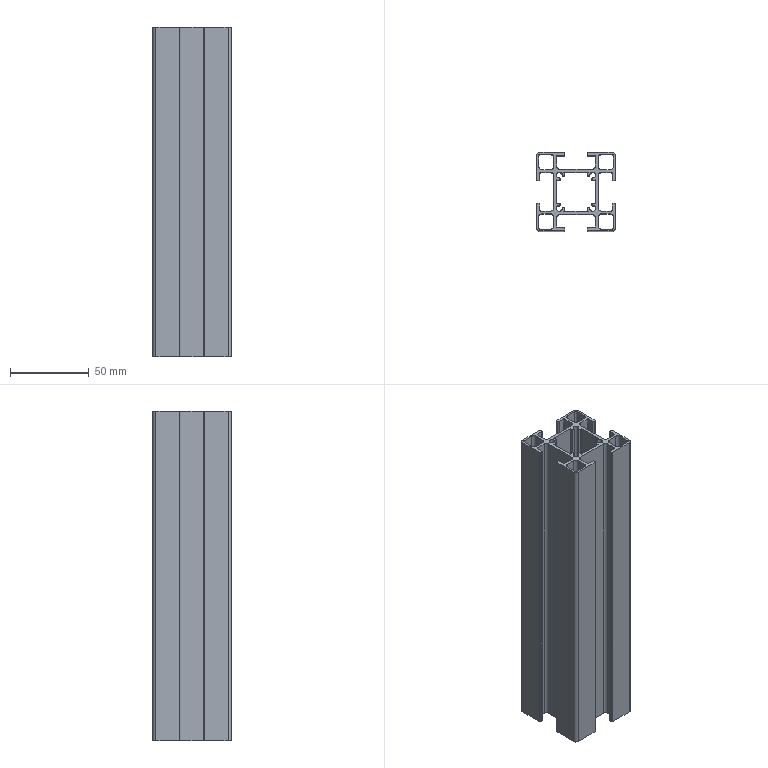Part | STEP file | 46A-00006CC11-210mm | 1 solid | 142 faces | box 50 x 50 x 210 mm | volume 123373 mm3 | cylinder 84 | plane 58 | commonest cylinder face diameters 1 x24 4 x24 1.5 x16 3.7 x8 6.7 x8 2 x4